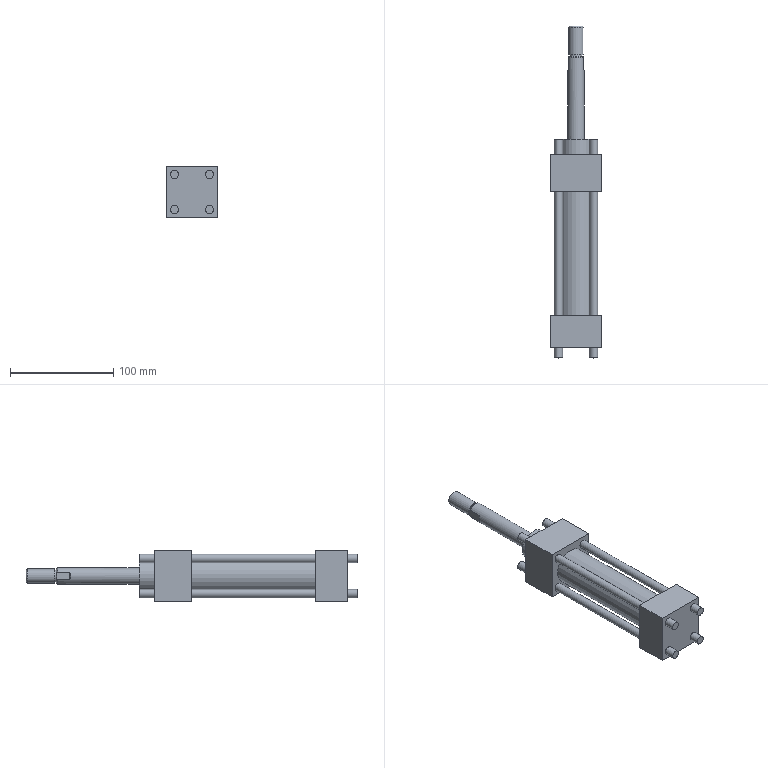Part | NX | features solid 2 | 1 solid | 52 faces | box 50 x 321.5 x 50 mm | volume 339915 mm3 | plane 28 | cylinder 19 | cone 5 | commonest cylinder face diameters 8 x12 15 x2 12 x1 14 x1 16 x1 30 x1
STEP:
#1=CARTESIAN_POINT('',(7.5,-465.5,-35.5));
#2=VERTEX_POINT('',#1);
#3=CARTESIAN_POINT('',(0.,-465.5,-35.5));
#4=DIRECTION('',(0.,0.,-1.));
#5=DIRECTION('',(1.,0.,0.));
#6=AXIS2_PLACEMENT_3D('',#3,#4,#5);
#7=CIRCLE('',#6,7.5);
#8=EDGE_CURVE('',#2,#2,#7,.F.);
#9=ORIENTED_EDGE('',*,*,#8,.T.);
#10=EDGE_LOOP('',(#9));
#11=FACE_BOUND('',#10,.T.);
#12=CARTESIAN_POINT('',(7.5,-465.5,-43.));
#13=VERTEX_POINT('',#12);
#14=CARTESIAN_POINT('',(0.,-465.5,-43.));
#15=DIRECTION('',(0.,0.,1.));
#16=DIRECTION('',(1.,0.,0.));
#17=AXIS2_PLACEMENT_3D('',#14,#15,#16);
#18=CIRCLE('',#17,7.5);
#19=EDGE_CURVE('',#13,#13,#18,.F.);
#20=ORIENTED_EDGE('',*,*,#19,.T.);
#21=EDGE_LOOP('',(#20));
#22=FACE_BOUND('',#21,.T.);
#23=CARTESIAN_POINT('',(0.,-465.5,-45.5));
#24=DIRECTION('',(0.,0.,1.));
#25=DIRECTION('',(1.,0.,0.));
#26=AXIS2_PLACEMENT_3D('',#23,#24,#25);
#27=CYLINDRICAL_SURFACE('',#26,7.5);
#28=ADVANCED_FACE('',(#11,#22),#27,.F.);
#29=CARTESIAN_POINT('',(7.5,-309.5,-35.5));
#30=VERTEX_POINT('',#29);
#31=CARTESIAN_POINT('',(0.,-309.5,-35.5));
#32=DIRECTION('',(0.,0.,-1.));
#33=DIRECTION('',(1.,0.,0.));
#34=AXIS2_PLACEMENT_3D('',#31,#32,#33);
#35=CIRCLE('',#34,7.5);
#36=EDGE_CURVE('',#30,#30,#35,.F.);
#37=ORIENTED_EDGE('',*,*,#36,.T.);
#38=EDGE_LOOP('',(#37));
#39=FACE_BOUND('',#38,.T.);
#40=CARTESIAN_POINT('',(7.5,-309.5,-43.));
#41=VERTEX_POINT('',#40);
#42=CARTESIAN_POINT('',(0.,-309.5,-43.));
#43=DIRECTION('',(0.,0.,1.));
#44=DIRECTION('',(1.,0.,0.));
#45=AXIS2_PLACEMENT_3D('',#42,#43,#44);
#46=CIRCLE('',#45,7.5);
#47=EDGE_CURVE('',#41,#41,#46,.F.);
#48=ORIENTED_EDGE('',*,*,#47,.T.);
#49=EDGE_LOOP('',(#48));
#50=FACE_BOUND('',#49,.T.);
#51=CARTESIAN_POINT('',(0.,-309.5,-45.5));
#52=DIRECTION('',(0.,0.,1.));
#53=DIRECTION('',(1.,0.,0.));
#54=AXIS2_PLACEMENT_3D('',#51,#52,#53);
#55=CYLINDRICAL_SURFACE('',#54,7.5);
#56=ADVANCED_FACE('',(#39,#50),#55,.F.);
#57=CARTESIAN_POINT('',(0.,-167.,-12.));
#58=VERTEX_POINT('',#57);
#59=CARTESIAN_POINT('',(0.,-167.,-18.));
#60=DIRECTION('',(0.,1.,0.));
#61=DIRECTION('',(0.,0.,1.));
#62=AXIS2_PLACEMENT_3D('',#59,#60,#61);
#63=CIRCLE('',#62,6.);
#64=EDGE_CURVE('',#58,#58,#63,.T.);
#65=ORIENTED_EDGE('',*,*,#64,.T.);
#66=EDGE_LOOP('',(#65));
#67=FACE_BOUND('',#66,.T.);
#68=CARTESIAN_POINT('',(0.,-167.,-18.));
#69=DIRECTION('',(0.,1.,0.));
#70=DIRECTION('',(0.,0.,-1.));
#71=AXIS2_PLACEMENT_3D('',#68,#69,#70);
#72=PLANE('',#71);
#73=ADVANCED_FACE('',(#67),#72,.T.);
#74=CARTESIAN_POINT('',(17.,-327.5,-5.));
#75=VERTEX_POINT('',#74);
#76=CARTESIAN_POINT('',(17.,-327.5,-1.));
#77=DIRECTION('',(0.,-1.,0.));
#78=DIRECTION('',(0.,0.,-1.));
#79=AXIS2_PLACEMENT_3D('',#76,#77,#78);
#80=CIRCLE('',#79,4.);
#81=EDGE_CURVE('',#75,#75,#80,.F.);
#82=ORIENTED_EDGE('',*,*,#81,.T.);
#83=EDGE_LOOP('',(#82));
#84=FACE_BOUND('',#83,.T.);
#85=CARTESIAN_POINT('',(17.,-327.5,-39.));
#86=VERTEX_POINT('',#85);
#87=CARTESIAN_POINT('',(17.,-327.5,-35.));
#88=DIRECTION('',(0.,-1.,0.));
#89=DIRECTION('',(0.,0.,-1.));
#90=AXIS2_PLACEMENT_3D('',#87,#88,#89);
#91=CIRCLE('',#90,4.);
#92=EDGE_CURVE('',#86,#86,#91,.F.);
#93=ORIENTED_EDGE('',*,*,#92,.T.);
#94=EDGE_LOOP('',(#93));
#95=FACE_BOUND('',#94,.T.);
#96=CARTESIAN_POINT('',(-17.,-327.5,-5.));
#97=VERTEX_POINT('',#96);
#98=CARTESIAN_POINT('',(-17.,-327.5,-1.));
#99=DIRECTION('',(0.,-1.,0.));
#100=DIRECTION('',(0.,0.,-1.));
#101=AXIS2_PLACEMENT_3D('',#98,#99,#100);
#102=CIRCLE('',#101,4.);
#103=EDGE_CURVE('',#97,#97,#102,.F.);
#104=ORIENTED_EDGE('',*,*,#103,.T.);
#105=EDGE_LOOP('',(#104));
#106=FACE_BOUND('',#105,.T.);
#107=CARTESIAN_POINT('',(-17.,-327.5,-39.));
#108=VERTEX_POINT('',#107);
#109=CARTESIAN_POINT('',(-17.,-327.5,-35.));
#110=DIRECTION('',(0.,-1.,0.));
#111=DIRECTION('',(0.,0.,-1.));
#112=AXIS2_PLACEMENT_3D('',#109,#110,#111);
#113=CIRCLE('',#112,4.);
#114=EDGE_CURVE('',#108,#108,#113,.T.);
#115=ORIENTED_EDGE('',*,*,#114,.F.);
#116=EDGE_LOOP('',(#115));
#117=FACE_BOUND('',#116,.T.);
#118=CARTESIAN_POINT('',(0.,-327.5,-35.5));
#119=VERTEX_POINT('',#118);
#120=CARTESIAN_POINT('',(0.,-327.5,-18.));
#121=DIRECTION('',(0.,-1.,0.));
#122=DIRECTION('',(0.,0.,-1.));
#123=AXIS2_PLACEMENT_3D('',#120,#121,#122);
#124=CIRCLE('',#123,17.5);
#125=EDGE_CURVE('',#119,#119,#124,.F.);
#126=ORIENTED_EDGE('',*,*,#125,.T.);
#127=EDGE_LOOP('',(#126));
#128=FACE_BOUND('',#127,.T.);
#129=CARTESIAN_POINT('',(-25.,-327.5,-43.));
#130=VERTEX_POINT('',#129);
#131=CARTESIAN_POINT('',(-25.,-327.5,7.));
#132=VERTEX_POINT('',#131);
#133=CARTESIAN_POINT('',(-25.,-327.5,9.5));
#134=DIRECTION('',(0.,0.,1.));
#135=VECTOR('',#134,1000.);
#136=LINE('',#133,#135);
#137=EDGE_CURVE('',#130,#132,#136,.T.);
#138=ORIENTED_EDGE('',*,*,#137,.F.);
#139=CARTESIAN_POINT('',(25.,-327.5,-43.));
#140=VERTEX_POINT('',#139);
#141=CARTESIAN_POINT('',(-27.5,-327.5,-43.));
#142=DIRECTION('',(-1.,0.,0.));
#143=VECTOR('',#142,1000.);
#144=LINE('',#141,#143);
#145=EDGE_CURVE('',#140,#130,#144,.T.);
#146=ORIENTED_EDGE('',*,*,#145,.F.);
#147=CARTESIAN_POINT('',(25.,-327.5,7.));
#148=VERTEX_POINT('',#147);
#149=CARTESIAN_POINT('',(25.,-327.5,9.5));
#150=DIRECTION('',(0.,0.,-1.));
#151=VECTOR('',#150,1000.);
#152=LINE('',#149,#151);
#153=EDGE_CURVE('',#148,#140,#152,.T.);
#154=ORIENTED_EDGE('',*,*,#153,.F.);
#155=CARTESIAN_POINT('',(-27.5,-327.5,7.));
#156=DIRECTION('',(1.,0.,0.));
#157=VECTOR('',#156,1000.);
#158=LINE('',#155,#157);
#159=EDGE_CURVE('',#132,#148,#158,.T.);
#160=ORIENTED_EDGE('',*,*,#159,.F.);
#161=EDGE_LOOP('',(#138,#146,#154,#160));
#162=FACE_BOUND('',#161,.T.);
#163=CARTESIAN_POINT('',(-27.5,-327.5,9.5));
#164=DIRECTION('',(0.,-1.,0.));
#165=DIRECTION('',(0.,0.,1.));
#166=AXIS2_PLACEMENT_3D('',#163,#164,#165);
#167=PLANE('',#166);
#168=ADVANCED_FACE('',(#84,#95,#106,#117,#128,#162),#167,.T.);
#169=CARTESIAN_POINT('',(0.,-291.5,-3.));
#170=VERTEX_POINT('',#169);
#171=CARTESIAN_POINT('',(0.,-291.5,-18.));
#172=DIRECTION('',(0.,1.,0.));
#173=DIRECTION('',(0.,0.,1.));
#174=AXIS2_PLACEMENT_3D('',#171,#172,#173);
#175=CIRCLE('',#174,15.);
#176=EDGE_CURVE('',#170,#170,#175,.T.);
#177=ORIENTED_EDGE('',*,*,#176,.F.);
#178=EDGE_LOOP('',(#177));
#179=FACE_BOUND('',#178,.T.);
#180=CARTESIAN_POINT('',(17.,-291.5,-5.));
#181=VERTEX_POINT('',#180);
#182=CARTESIAN_POINT('',(17.,-291.5,-1.));
#183=DIRECTION('',(0.,-1.,0.));
#184=DIRECTION('',(0.,0.,-1.));
#185=AXIS2_PLACEMENT_3D('',#182,#183,#184);
#186=CIRCLE('',#185,4.);
#187=EDGE_CURVE('',#181,#181,#186,.F.);
#188=ORIENTED_EDGE('',*,*,#187,.F.);
#189=EDGE_LOOP('',(#188));
#190=FACE_BOUND('',#189,.T.);
#191=CARTESIAN_POINT('',(17.,-291.5,-39.));
#192=VERTEX_POINT('',#191);
#193=CARTESIAN_POINT('',(17.,-291.5,-35.));
#194=DIRECTION('',(0.,-1.,0.));
#195=DIRECTION('',(0.,0.,-1.));
#196=AXIS2_PLACEMENT_3D('',#193,#194,#195);
#197=CIRCLE('',#196,4.);
#198=EDGE_CURVE('',#192,#192,#197,.F.);
#199=ORIENTED_EDGE('',*,*,#198,.F.);
#200=EDGE_LOOP('',(#199));
#201=FACE_BOUND('',#200,.T.);
#202=CARTESIAN_POINT('',(-17.,-291.5,-5.));
#203=VERTEX_POINT('',#202);
#204=CARTESIAN_POINT('',(-17.,-291.5,-1.));
#205=DIRECTION('',(0.,-1.,0.));
#206=DIRECTION('',(0.,0.,-1.));
#207=AXIS2_PLACEMENT_3D('',#204,#205,#206);
#208=CIRCLE('',#207,4.);
#209=EDGE_CURVE('',#203,#203,#208,.F.);
#210=ORIENTED_EDGE('',*,*,#209,.F.);
#211=EDGE_LOOP('',(#210));
#212=FACE_BOUND('',#211,.T.);
#213=CARTESIAN_POINT('',(-17.,-291.5,-39.));
#214=VERTEX_POINT('',#213);
#215=CARTESIAN_POINT('',(-17.,-291.5,-35.));
#216=DIRECTION('',(0.,-1.,0.));
#217=DIRECTION('',(0.,0.,-1.));
#218=AXIS2_PLACEMENT_3D('',#215,#216,#217);
#219=CIRCLE('',#218,4.);
#220=EDGE_CURVE('',#214,#214,#219,.T.);
#221=ORIENTED_EDGE('',*,*,#220,.T.);
#222=EDGE_LOOP('',(#221));
#223=FACE_BOUND('',#222,.T.);
#224=CARTESIAN_POINT('',(-25.,-291.5,-43.));
#225=VERTEX_POINT('',#224);
#226=CARTESIAN_POINT('',(-25.,-291.5,7.));
#227=VERTEX_POINT('',#226);
#228=CARTESIAN_POINT('',(-25.,-291.5,9.5));
#229=DIRECTION('',(0.,0.,1.));
#230=VECTOR('',#229,1000.);
#231=LINE('',#228,#230);
#232=EDGE_CURVE('',#225,#227,#231,.T.);
#233=ORIENTED_EDGE('',*,*,#232,.T.);
#234=CARTESIAN_POINT('',(25.,-291.5,7.));
#235=VERTEX_POINT('',#234);
#236=CARTESIAN_POINT('',(-27.5,-291.5,7.));
#237=DIRECTION('',(1.,0.,0.));
#238=VECTOR('',#237,1000.);
#239=LINE('',#236,#238);
#240=EDGE_CURVE('',#227,#235,#239,.T.);
#241=ORIENTED_EDGE('',*,*,#240,.T.);
#242=CARTESIAN_POINT('',(25.,-291.5,-43.));
#243=VERTEX_POINT('',#242);
#244=CARTESIAN_POINT('',(25.,-291.5,9.5));
#245=DIRECTION('',(0.,0.,-1.));
#246=VECTOR('',#245,1000.);
#247=LINE('',#244,#246);
#248=EDGE_CURVE('',#235,#243,#247,.T.);
#249=ORIENTED_EDGE('',*,*,#248,.T.);
#250=CARTESIAN_POINT('',(-27.5,-291.5,-43.));
#251=DIRECTION('',(-1.,0.,0.));
#252=VECTOR('',#251,1000.);
#253=LINE('',#250,#252);
#254=EDGE_CURVE('',#243,#225,#253,.T.);
#255=ORIENTED_EDGE('',*,*,#254,.T.);
#256=EDGE_LOOP('',(#233,#241,#249,#255));
#257=FACE_BOUND('',#256,.T.);
#258=CARTESIAN_POINT('',(-27.5,-291.5,9.5));
#259=DIRECTION('',(0.,-1.,0.));
#260=DIRECTION('',(0.,0.,1.));
#261=AXIS2_PLACEMENT_3D('',#258,#259,#260);
#262=PLANE('',#261);
#263=ADVANCED_FACE('',(#179,#190,#201,#212,#223,#257),#262,.F.);
#264=ORIENTED_EDGE('',*,*,#232,.F.);
#265=CARTESIAN_POINT('',(-25.,-327.5,-43.));
#266=DIRECTION('',(0.,1.,0.));
#267=VECTOR('',#266,1000.);
#268=LINE('',#265,#267);
#269=EDGE_CURVE('',#130,#225,#268,.T.);
#270=ORIENTED_EDGE('',*,*,#269,.F.);
#271=ORIENTED_EDGE('',*,*,#137,.T.);
#272=CARTESIAN_POINT('',(-25.,-327.5,7.));
#273=DIRECTION('',(0.,1.,0.));
#274=VECTOR('',#273,1000.);
#275=LINE('',#272,#274);
#276=EDGE_CURVE('',#132,#227,#275,.T.);
#277=ORIENTED_EDGE('',*,*,#276,.T.);
#278=EDGE_LOOP('',(#264,#270,#271,#277));
#279=FACE_BOUND('',#278,.T.);
#280=CARTESIAN_POINT('',(-25.,-327.5,-45.5));
#281=DIRECTION('',(1.,0.,0.));
#282=DIRECTION('',(0.,0.,-1.));
#283=AXIS2_PLACEMENT_3D('',#280,#281,#282);
#284=PLANE('',#283);
#285=ADVANCED_FACE('',(#279),#284,.F.);
#286=ORIENTED_EDGE('',*,*,#240,.F.);
#287=ORIENTED_EDGE('',*,*,#276,.F.);
#288=ORIENTED_EDGE('',*,*,#159,.T.);
#289=CARTESIAN_POINT('',(25.,-327.5,7.));
#290=DIRECTION('',(0.,1.,0.));
#291=VECTOR('',#290,1000.);
#292=LINE('',#289,#291);
#293=EDGE_CURVE('',#148,#235,#292,.T.);
#294=ORIENTED_EDGE('',*,*,#293,.T.);
#295=EDGE_LOOP('',(#286,#287,#288,#294));
#296=FACE_BOUND('',#295,.T.);
#297=CARTESIAN_POINT('',(-27.5,-327.5,7.));
#298=DIRECTION('',(0.,0.,-1.));
#299=DIRECTION('',(0.,-1.,0.));
#300=AXIS2_PLACEMENT_3D('',#297,#298,#299);
#301=PLANE('',#300);
#302=ADVANCED_FACE('',(#296),#301,.F.);
#303=ORIENTED_EDGE('',*,*,#248,.F.);
#304=ORIENTED_EDGE('',*,*,#293,.F.);
#305=ORIENTED_EDGE('',*,*,#153,.T.);
#306=CARTESIAN_POINT('',(25.,-327.5,-43.));
#307=DIRECTION('',(0.,1.,0.));
#308=VECTOR('',#307,1000.);
#309=LINE('',#306,#308);
#310=EDGE_CURVE('',#140,#243,#309,.T.);
#311=ORIENTED_EDGE('',*,*,#310,.T.);
#312=EDGE_LOOP('',(#303,#304,#305,#311));
#313=FACE_BOUND('',#312,.T.);
#314=CARTESIAN_POINT('',(25.,-327.5,9.5));
#315=DIRECTION('',(-1.,0.,0.));
#316=DIRECTION('',(0.,0.,1.));
#317=AXIS2_PLACEMENT_3D('',#314,#315,#316);
#318=PLANE('',#317);
#319=ADVANCED_FACE('',(#313),#318,.F.);
#320=ORIENTED_EDGE('',*,*,#47,.F.);
#321=EDGE_LOOP('',(#320));
#322=FACE_BOUND('',#321,.T.);
#323=ORIENTED_EDGE('',*,*,#254,.F.);
#324=ORIENTED_EDGE('',*,*,#310,.F.);
#325=ORIENTED_EDGE('',*,*,#145,.T.);
#326=ORIENTED_EDGE('',*,*,#269,.T.);
#327=EDGE_LOOP('',(#323,#324,#325,#326));
#328=FACE_BOUND('',#327,.T.);
#329=CARTESIAN_POINT('',(27.5,-327.5,-43.));
#330=DIRECTION('',(0.,0.,1.));
#331=DIRECTION('',(1.,0.,0.));
#332=AXIS2_PLACEMENT_3D('',#329,#330,#331);
#333=PLANE('',#332);
#334=ADVANCED_FACE('',(#322,#328),#333,.F.);
#335=CARTESIAN_POINT('',(0.,-447.5,-35.5));
#336=VERTEX_POINT('',#335);
#337=CARTESIAN_POINT('',(0.,-447.5,-18.));
#338=DIRECTION('',(0.,-1.,0.));
#339=DIRECTION('',(0.,0.,-1.));
#340=AXIS2_PLACEMENT_3D('',#337,#338,#339);
#341=CIRCLE('',#340,17.5);
#342=EDGE_CURVE('',#336,#336,#341,.F.);
#343=ORIENTED_EDGE('',*,*,#342,.T.);
#344=EDGE_LOOP('',(#343));
#345=FACE_BOUND('',#344,.T.);
#346=ORIENTED_EDGE('',*,*,#125,.F.);
#347=EDGE_LOOP('',(#346));
#348=FACE_BOUND('',#347,.T.);
#349=CARTESIAN_POINT('',(0.,-447.5,-18.));
#350=DIRECTION('',(0.,1.,0.));
#351=DIRECTION('',(0.,0.,-1.));
#352=AXIS2_PLACEMENT_3D('',#349,#350,#351);
#353=CYLINDRICAL_SURFACE('',#352,17.5);
#354=ADVANCED_FACE('',(#345,#348),#353,.T.);
#355=ORIENTED_EDGE('',*,*,#36,.F.);
#356=EDGE_LOOP('',(#355));
#357=FACE_BOUND('',#356,.T.);
#358=CARTESIAN_POINT('',(0.,-309.5,-30.994));
#359=VERTEX_POINT('',#358);
#360=VERTEX_LOOP('',#359);
#361=FACE_BOUND('',#360,.T.);
#362=CARTESIAN_POINT('',(0.,-309.5,-35.5));
#363=DIRECTION('',(0.,0.,-1.));
#364=DIRECTION('',(-1.,0.,0.));
#365=AXIS2_PLACEMENT_3D('',#362,#363,#364);
#366=CONICAL_SURFACE('',#365,7.5,1.03);
#367=ADVANCED_FACE('',(#357,#361),#366,.F.);
#368=CARTESIAN_POINT('',(17.,-447.5,-5.));
#369=VERTEX_POINT('',#368);
#370=CARTESIAN_POINT('',(17.,-447.5,-1.));
#371=DIRECTION('',(0.,-1.,0.));
#372=DIRECTION('',(0.,0.,-1.));
#373=AXIS2_PLACEMENT_3D('',#370,#371,#372);
#374=CIRCLE('',#373,4.);
#375=EDGE_CURVE('',#369,#369,#374,.F.);
#376=ORIENTED_EDGE('',*,*,#375,.F.);
#377=EDGE_LOOP('',(#376));
#378=FACE_BOUND('',#377,.T.);
#379=CARTESIAN_POINT('',(17.,-447.5,-39.));
#380=VERTEX_POINT('',#379);
#381=CARTESIAN_POINT('',(17.,-447.5,-35.));
#382=DIRECTION('',(0.,-1.,0.));
#383=DIRECTION('',(0.,0.,-1.));
#384=AXIS2_PLACEMENT_3D('',#381,#382,#383);
#385=CIRCLE('',#384,4.);
#386=EDGE_CURVE('',#380,#380,#385,.F.);
#387=ORIENTED_EDGE('',*,*,#386,.F.);
#388=EDGE_LOOP('',(#387));
#389=FACE_BOUND('',#388,.T.);
#390=CARTESIAN_POINT('',(-17.,-447.5,-5.));
#391=VERTEX_POINT('',#390);
#392=CARTESIAN_POINT('',(-17.,-447.5,-1.));
#393=DIRECTION('',(0.,-1.,0.));
#394=DIRECTION('',(0.,0.,-1.));
#395=AXIS2_PLACEMENT_3D('',#392,#393,#394);
#396=CIRCLE('',#395,4.);
#397=EDGE_CURVE('',#391,#391,#396,.F.);
#398=ORIENTED_EDGE('',*,*,#397,.F.);
#399=EDGE_LOOP('',(#398));
#400=FACE_BOUND('',#399,.T.);
#401=CARTESIAN_POINT('',(-17.,-447.5,-39.));
#402=VERTEX_POINT('',#401);
#403=CARTESIAN_POINT('',(-17.,-447.5,-35.));
#404=DIRECTION('',(0.,-1.,0.));
#405=DIRECTION('',(0.,0.,-1.));
#406=AXIS2_PLACEMENT_3D('',#403,#404,#405);
#407=CIRCLE('',#406,4.);
#408=EDGE_CURVE('',#402,#402,#407,.T.);
#409=ORIENTED_EDGE('',*,*,#408,.T.);
#410=EDGE_LOOP('',(#409));
#411=FACE_BOUND('',#410,.T.);
#412=CARTESIAN_POINT('',(-25.,-447.5,-43.));
#413=VERTEX_POINT('',#412);
#414=CARTESIAN_POINT('',(-25.,-447.5,7.));
#415=VERTEX_POINT('',#414);
#416=CARTESIAN_POINT('',(-25.,-447.5,9.5));
#417=DIRECTION('',(0.,0.,1.));
#418=VECTOR('',#417,1000.);
#419=LINE('',#416,#418);
#420=EDGE_CURVE('',#413,#415,#419,.T.);
#421=ORIENTED_EDGE('',*,*,#420,.T.);
#422=CARTESIAN_POINT('',(25.,-447.5,7.));
#423=VERTEX_POINT('',#422);
#424=CARTESIAN_POINT('',(-27.5,-447.5,7.));
#425=DIRECTION('',(1.,0.,0.));
#426=VECTOR('',#425,1000.);
#427=LINE('',#424,#426);
#428=EDGE_CURVE('',#415,#423,#427,.T.);
#429=ORIENTED_EDGE('',*,*,#428,.T.);
#430=CARTESIAN_POINT('',(25.,-447.5,-43.));
#431=VERTEX_POINT('',#430);
#432=CARTESIAN_POINT('',(25.,-447.5,9.5));
#433=DIRECTION('',(0.,0.,-1.));
#434=VECTOR('',#433,1000.);
#435=LINE('',#432,#434);
#436=EDGE_CURVE('',#423,#431,#435,.T.);
#437=ORIENTED_EDGE('',*,*,#436,.T.);
#438=CARTESIAN_POINT('',(-27.5,-447.5,-43.));
#439=DIRECTION('',(-1.,0.,0.));
#440=VECTOR('',#439,1000.);
#441=LINE('',#438,#440);
#442=EDGE_CURVE('',#431,#413,#441,.T.);
#443=ORIENTED_EDGE('',*,*,#442,.T.);
#444=EDGE_LOOP('',(#421,#429,#437,#443));
#445=FACE_BOUND('',#444,.T.);
#446=ORIENTED_EDGE('',*,*,#342,.F.);
#447=EDGE_LOOP('',(#446));
#448=FACE_BOUND('',#447,.T.);
#449=CARTESIAN_POINT('',(-27.5,-447.5,9.5));
#450=DIRECTION('',(0.,-1.,0.));
#451=DIRECTION('',(0.,0.,1.));
#452=AXIS2_PLACEMENT_3D('',#449,#450,#451);
#453=PLANE('',#452);
#454=ADVANCED_FACE('',(#378,#389,#400,#411,#445,#448),#453,.F.);
#455=CARTESIAN_POINT('',(17.,-478.5,-5.));
#456=VERTEX_POINT('',#455);
#457=CARTESIAN_POINT('',(17.,-478.5,-1.));
#458=DIRECTION('',(0.,-1.,0.));
#459=DIRECTION('',(0.,0.,-1.));
#460=AXIS2_PLACEMENT_3D('',#457,#458,#459);
#461=CIRCLE('',#460,4.);
#462=EDGE_CURVE('',#456,#456,#461,.F.);
#463=ORIENTED_EDGE('',*,*,#462,.T.);
#464=EDGE_LOOP('',(#463));
#465=FACE_BOUND('',#464,.T.);
#466=CARTESIAN_POINT('',(17.,-478.5,-39.));
#467=VERTEX_POINT('',#466);
#468=CARTESIAN_POINT('',(17.,-478.5,-35.));
#469=DIRECTION('',(0.,-1.,0.));
#470=DIRECTION('',(0.,0.,-1.));
#471=AXIS2_PLACEMENT_3D('',#468,#469,#470);
#472=CIRCLE('',#471,4.);
#473=EDGE_CURVE('',#467,#467,#472,.F.);
#474=ORIENTED_EDGE('',*,*,#473,.T.);
#475=EDGE_LOOP('',(#474));
#476=FACE_BOUND('',#475,.T.);
#477=CARTESIAN_POINT('',(-17.,-478.5,-5.));
#478=VERTEX_POINT('',#477);
#479=CARTESIAN_POINT('',(-17.,-478.5,-1.));
#480=DIRECTION('',(0.,-1.,0.));
#481=DIRECTION('',(0.,0.,-1.));
#482=AXIS2_PLACEMENT_3D('',#479,#480,#481);
#483=CIRCLE('',#482,4.);
#484=EDGE_CURVE('',#478,#478,#483,.F.);
#485=ORIENTED_EDGE('',*,*,#484,.T.);
#486=EDGE_LOOP('',(#485));
#487=FACE_BOUND('',#486,.T.);
#488=CARTESIAN_POINT('',(-17.,-478.5,-39.));
#489=VERTEX_POINT('',#488);
#490=CARTESIAN_POINT('',(-17.,-478.5,-35.));
#491=DIRECTION('',(0.,-1.,0.));
#492=DIRECTION('',(0.,0.,-1.));
#493=AXIS2_PLACEMENT_3D('',#490,#491,#492);
#494=CIRCLE('',#493,4.);
#495=EDGE_CURVE('',#489,#489,#494,.T.);
#496=ORIENTED_EDGE('',*,*,#495,.F.);
#497=EDGE_LOOP('',(#496));
#498=FACE_BOUND('',#497,.T.);
#499=CARTESIAN_POINT('',(25.,-478.5,7.));
#500=VERTEX_POINT('',#499);
#501=CARTESIAN_POINT('',(25.,-478.5,-43.));
#502=VERTEX_POINT('',#501);
#503=CARTESIAN_POINT('',(25.,-478.5,9.5));
#504=DIRECTION('',(0.,0.,-1.));
#505=VECTOR('',#504,1000.);
#506=LINE('',#503,#505);
#507=EDGE_CURVE('',#500,#502,#506,.T.);
#508=ORIENTED_EDGE('',*,*,#507,.F.);
#509=CARTESIAN_POINT('',(-25.,-478.5,7.));
#510=VERTEX_POINT('',#509);
#511=CARTESIAN_POINT('',(-27.5,-478.5,7.));
#512=DIRECTION('',(1.,0.,0.));
#513=VECTOR('',#512,1000.);
#514=LINE('',#511,#513);
#515=EDGE_CURVE('',#510,#500,#514,.T.);
#516=ORIENTED_EDGE('',*,*,#515,.F.);
#517=CARTESIAN_POINT('',(-25.,-478.5,-43.));
#518=VERTEX_POINT('',#517);
#519=CARTESIAN_POINT('',(-25.,-478.5,9.5));
#520=DIRECTION('',(0.,0.,1.));
#521=VECTOR('',#520,1000.);
#522=LINE('',#519,#521);
#523=EDGE_CURVE('',#518,#510,#522,.T.);
#524=ORIENTED_EDGE('',*,*,#523,.F.);
#525=CARTESIAN_POINT('',(-27.5,-478.5,-43.));
#526=DIRECTION('',(-1.,0.,0.));
#527=VECTOR('',#526,1000.);
#528=LINE('',#525,#527);
#529=EDGE_CURVE('',#502,#518,#528,.T.);
#530=ORIENTED_EDGE('',*,*,#529,.F.);
#531=EDGE_LOOP('',(#508,#516,#524,#530));
#532=FACE_BOUND('',#531,.T.);
#533=CARTESIAN_POINT('',(-27.5,-478.5,9.5));
#534=DIRECTION('',(0.,-1.,0.));
#535=DIRECTION('',(0.,0.,1.));
#536=AXIS2_PLACEMENT_3D('',#533,#534,#535);
#537=PLANE('',#536);
#538=ADVANCED_FACE('',(#465,#476,#487,#498,#532),#537,.T.);
#539=ORIENTED_EDGE('',*,*,#420,.F.);
#540=CARTESIAN_POINT('',(-25.,-478.5,-43.));
#541=DIRECTION('',(0.,1.,0.));
#542=VECTOR('',#541,1000.);
#543=LINE('',#540,#542);
#544=EDGE_CURVE('',#518,#413,#543,.T.);
#545=ORIENTED_EDGE('',*,*,#544,.F.);
#546=ORIENTED_EDGE('',*,*,#523,.T.);
#547=CARTESIAN_POINT('',(-25.,-478.5,7.));
#548=DIRECTION('',(0.,1.,0.));
#549=VECTOR('',#548,1000.);
#550=LINE('',#547,#549);
#551=EDGE_CURVE('',#510,#415,#550,.T.);
#552=ORIENTED_EDGE('',*,*,#551,.T.);
#553=EDGE_LOOP('',(#539,#545,#546,#552));
#554=FACE_BOUND('',#553,.T.);
#555=CARTESIAN_POINT('',(-25.,-478.5,-45.5));
#556=DIRECTION('',(1.,0.,0.));
#557=DIRECTION('',(0.,0.,-1.));
#558=AXIS2_PLACEMENT_3D('',#555,#556,#557);
#559=PLANE('',#558);
#560=ADVANCED_FACE('',(#554),#559,.F.);
#561=ORIENTED_EDGE('',*,*,#428,.F.);
#562=ORIENTED_EDGE('',*,*,#551,.F.);
#563=ORIENTED_EDGE('',*,*,#515,.T.);
#564=CARTESIAN_POINT('',(25.,-478.5,7.));
#565=DIRECTION('',(0.,1.,0.));
#566=VECTOR('',#565,1000.);
#567=LINE('',#564,#566);
#568=EDGE_CURVE('',#500,#423,#567,.T.);
#569=ORIENTED_EDGE('',*,*,#568,.T.);
#570=EDGE_LOOP('',(#561,#562,#563,#569));
#571=FACE_BOUND('',#570,.T.);
#572=CARTESIAN_POINT('',(-27.5,-478.5,7.));
#573=DIRECTION('',(0.,0.,-1.));
#574=DIRECTION('',(-1.,0.,0.));
#575=AXIS2_PLACEMENT_3D('',#572,#573,#574);
#576=PLANE('',#575);
#577=ADVANCED_FACE('',(#571),#576,.F.);
#578=ORIENTED_EDGE('',*,*,#436,.F.);
#579=ORIENTED_EDGE('',*,*,#568,.F.);
#580=ORIENTED_EDGE('',*,*,#507,.T.);
#581=CARTESIAN_POINT('',(25.,-478.5,-43.));
#582=DIRECTION('',(0.,1.,0.));
#583=VECTOR('',#582,1000.);
#584=LINE('',#581,#583);
#585=EDGE_CURVE('',#502,#431,#584,.T.);
#586=ORIENTED_EDGE('',*,*,#585,.T.);
#587=EDGE_LOOP('',(#578,#579,#580,#586));
#588=FACE_BOUND('',#587,.T.);
#589=CARTESIAN_POINT('',(25.,-478.5,9.5));
#590=DIRECTION('',(-1.,0.,0.));
#591=DIRECTION('',(0.,0.,1.));
#592=AXIS2_PLACEMENT_3D('',#589,#590,#591);
#593=PLANE('',#592);
#594=ADVANCED_FACE('',(#588),#593,.F.);
#595=ORIENTED_EDGE('',*,*,#19,.F.);
#596=EDGE_LOOP('',(#595));
#597=FACE_BOUND('',#596,.T.);
#598=ORIENTED_EDGE('',*,*,#442,.F.);
#599=ORIENTED_EDGE('',*,*,#585,.F.);
#600=ORIENTED_EDGE('',*,*,#529,.T.);
#601=ORIENTED_EDGE('',*,*,#544,.T.);
#602=EDGE_LOOP('',(#598,#599,#600,#601));
#603=FACE_BOUND('',#602,.T.);
#604=CARTESIAN_POINT('',(27.5,-478.5,-43.));
#605=DIRECTION('',(0.,0.,1.));
#606=DIRECTION('',(1.,0.,0.));
#607=AXIS2_PLACEMENT_3D('',#604,#605,#606);
#608=PLANE('',#607);
#609=ADVANCED_FACE('',(#597,#603),#608,.F.);
#610=ORIENTED_EDGE('',*,*,#8,.F.);
#611=EDGE_LOOP('',(#610));
#612=FACE_BOUND('',#611,.T.);
#613=CARTESIAN_POINT('',(0.,-465.5,-30.994));
#614=VERTEX_POINT('',#613);
#615=VERTEX_LOOP('',#614);
#616=FACE_BOUND('',#615,.T.);
#617=CARTESIAN_POINT('',(0.,-465.5,-35.5));
#618=DIRECTION('',(0.,0.,-1.));
#619=DIRECTION('',(-1.,0.,0.));
#620=AXIS2_PLACEMENT_3D('',#617,#618,#619);
#621=CONICAL_SURFACE('',#620,7.5,1.03);
#622=ADVANCED_FACE('',(#612,#616),#621,.F.);
#623=CARTESIAN_POINT('',(-17.,-488.5,-31.));
#624=VERTEX_POINT('',#623);
#625=CARTESIAN_POINT('',(-17.,-488.5,-35.));
#626=DIRECTION('',(0.,1.,0.));
#627=DIRECTION('',(0.,0.,1.));
#628=AXIS2_PLACEMENT_3D('',#625,#626,#627);
#629=CIRCLE('',#628,4.);
#630=EDGE_CURVE('',#624,#624,#629,.T.);
#631=ORIENTED_EDGE('',*,*,#630,.F.);
#632=EDGE_LOOP('',(#631));
#633=FACE_BOUND('',#632,.T.);
#634=CARTESIAN_POINT('',(20.,-488.5,-38.));
#635=DIRECTION('',(0.,1.,0.));
#636=DIRECTION('',(0.,0.,-1.));
#637=AXIS2_PLACEMENT_3D('',#634,#635,#636);
#638=PLANE('',#637);
#639=ADVANCED_FACE('',(#633),#638,.F.);
#640=ORIENTED_EDGE('',*,*,#495,.T.);
#641=EDGE_LOOP('',(#640));
#642=FACE_BOUND('',#641,.T.);
#643=ORIENTED_EDGE('',*,*,#630,.T.);
#644=EDGE_LOOP('',(#643));
#645=FACE_BOUND('',#644,.T.);
#646=CARTESIAN_POINT('',(-17.,-561.5,-35.));
#647=DIRECTION('',(0.,1.,0.));
#648=DIRECTION('',(0.,0.,1.));
#649=AXIS2_PLACEMENT_3D('',#646,#647,#648);
#650=CYLINDRICAL_SURFACE('',#649,4.);
#651=ADVANCED_FACE('',(#642,#645),#650,.T.);
#652=ORIENTED_EDGE('',*,*,#114,.T.);
#653=EDGE_LOOP('',(#652));
#654=FACE_BOUND('',#653,.T.);
#655=ORIENTED_EDGE('',*,*,#408,.F.);
#656=EDGE_LOOP('',(#655));
#657=FACE_BOUND('',#656,.T.);
#658=CARTESIAN_POINT('',(-17.,-556.5,-35.));
#659=DIRECTION('',(0.,1.,0.));
#660=DIRECTION('',(0.,0.,1.));
#661=AXIS2_PLACEMENT_3D('',#658,#659,#660);
#662=CYLINDRICAL_SURFACE('',#661,4.);
#663=ADVANCED_FACE('',(#654,#657),#662,.T.);
#664=CARTESIAN_POINT('',(-17.,-276.5,-31.));
#665=VERTEX_POINT('',#664);
#666=CARTESIAN_POINT('',(-17.,-276.5,-35.));
#667=DIRECTION('',(0.,1.,0.));
#668=DIRECTION('',(0.,0.,1.));
#669=AXIS2_PLACEMENT_3D('',#666,#667,#668);
#670=CIRCLE('',#669,4.);
#671=EDGE_CURVE('',#665,#665,#670,.T.);
#672=ORIENTED_EDGE('',*,*,#671,.F.);
#673=EDGE_LOOP('',(#672));
#674=FACE_BOUND('',#673,.T.);
#675=ORIENTED_EDGE('',*,*,#220,.F.);
#676=EDGE_LOOP('',(#675));
#677=FACE_BOUND('',#676,.T.);
#678=CARTESIAN_POINT('',(-17.,-556.5,-35.));
#679=DIRECTION('',(0.,1.,0.));
#680=DIRECTION('',(0.,0.,1.));
#681=AXIS2_PLACEMENT_3D('',#678,#679,#680);
#682=CYLINDRICAL_SURFACE('',#681,4.);
#683=ADVANCED_FACE('',(#674,#677),#682,.T.);
#684=ORIENTED_EDGE('',*,*,#671,.T.);
#685=EDGE_LOOP('',(#684));
#686=FACE_BOUND('',#685,.T.);
#687=CARTESIAN_POINT('',(-17.,-276.5,-35.));
#688=DIRECTION('',(0.,1.,0.));
#689=DIRECTION('',(0.,0.,1.));
#690=AXIS2_PLACEMENT_3D('',#687,#688,#689);
#691=PLANE('',#690);
#692=ADVANCED_FACE('',(#686),#691,.T.);
#693=CARTESIAN_POINT('',(-17.,-488.5,3.));
#694=VERTEX_POINT('',#693);
#695=CARTESIAN_POINT('',(-17.,-488.5,-1.));
#696=DIRECTION('',(0.,1.,0.));
#697=DIRECTION('',(0.,0.,1.));
#698=AXIS2_PLACEMENT_3D('',#695,#696,#697);
#699=CIRCLE('',#698,4.);
#700=EDGE_CURVE('',#694,#694,#699,.F.);
#701=ORIENTED_EDGE('',*,*,#700,.T.);
#702=EDGE_LOOP('',(#701));
#703=FACE_BOUND('',#702,.T.);
#704=CARTESIAN_POINT('',(20.,-488.5,-38.));
#705=DIRECTION('',(0.,1.,0.));
#706=DIRECTION('',(0.,0.,-1.));
#707=AXIS2_PLACEMENT_3D('',#704,#705,#706);
#708=PLANE('',#707);
#709=ADVANCED_FACE('',(#703),#708,.F.);
#710=ORIENTED_EDGE('',*,*,#484,.F.);
#711=EDGE_LOOP('',(#710));
#712=FACE_BOUND('',#711,.T.);
#713=ORIENTED_EDGE('',*,*,#700,.F.);
#714=EDGE_LOOP('',(#713));
#715=FACE_BOUND('',#714,.T.);
#716=CARTESIAN_POINT('',(-17.,-561.5,-1.));
#717=DIRECTION('',(0.,1.,0.));
#718=DIRECTION('',(0.,0.,1.));
#719=AXIS2_PLACEMENT_3D('',#716,#717,#718);
#720=CYLINDRICAL_SURFACE('',#719,4.);
#721=ADVANCED_FACE('',(#712,#715),#720,.T.);
#722=ORIENTED_EDGE('',*,*,#103,.F.);
#723=EDGE_LOOP('',(#722));
#724=FACE_BOUND('',#723,.T.);
#725=ORIENTED_EDGE('',*,*,#397,.T.);
#726=EDGE_LOOP('',(#725));
#727=FACE_BOUND('',#726,.T.);
#728=CARTESIAN_POINT('',(-17.,-556.5,-1.));
#729=DIRECTION('',(0.,1.,0.));
#730=DIRECTION('',(0.,0.,1.));
#731=AXIS2_PLACEMENT_3D('',#728,#729,#730);
#732=CYLINDRICAL_SURFACE('',#731,4.);
#733=ADVANCED_FACE('',(#724,#727),#732,.T.);
#734=CARTESIAN_POINT('',(-17.,-276.5,-5.));
#735=VERTEX_POINT('',#734);
#736=CARTESIAN_POINT('',(-17.,-276.5,-1.));
#737=DIRECTION('',(0.,-1.,0.));
#738=DIRECTION('',(0.,0.,-1.));
#739=AXIS2_PLACEMENT_3D('',#736,#737,#738);
#740=CIRCLE('',#739,4.);
#741=EDGE_CURVE('',#735,#735,#740,.T.);
#742=ORIENTED_EDGE('',*,*,#741,.T.);
#743=EDGE_LOOP('',(#742));
#744=FACE_BOUND('',#743,.T.);
#745=ORIENTED_EDGE('',*,*,#209,.T.);
#746=EDGE_LOOP('',(#745));
#747=FACE_BOUND('',#746,.T.);
#748=CARTESIAN_POINT('',(-17.,-556.5,-1.));
#749=DIRECTION('',(0.,1.,0.));
#750=DIRECTION('',(0.,0.,1.));
#751=AXIS2_PLACEMENT_3D('',#748,#749,#750);
#752=CYLINDRICAL_SURFACE('',#751,4.);
#753=ADVANCED_FACE('',(#744,#747),#752,.T.);
#754=ORIENTED_EDGE('',*,*,#741,.F.);
#755=EDGE_LOOP('',(#754));
#756=FACE_BOUND('',#755,.T.);
#757=CARTESIAN_POINT('',(-17.,-276.5,-1.));
#758=DIRECTION('',(0.,-1.,0.));
#759=DIRECTION('',(0.,0.,-1.));
#760=AXIS2_PLACEMENT_3D('',#757,#758,#759);
#761=PLANE('',#760);
#762=ADVANCED_FACE('',(#756),#761,.F.);
#763=CARTESIAN_POINT('',(17.,-488.5,-39.));
#764=VERTEX_POINT('',#763);
#765=CARTESIAN_POINT('',(17.,-488.5,-35.));
#766=DIRECTION('',(0.,-1.,0.));
#767=DIRECTION('',(0.,0.,-1.));
#768=AXIS2_PLACEMENT_3D('',#765,#766,#767);
#769=CIRCLE('',#768,4.);
#770=EDGE_CURVE('',#764,#764,#769,.T.);
#771=ORIENTED_EDGE('',*,*,#770,.T.);
#772=EDGE_LOOP('',(#771));
#773=FACE_BOUND('',#772,.T.);
#774=CARTESIAN_POINT('',(20.,-488.5,2.));
#775=DIRECTION('',(0.,-1.,0.));
#776=DIRECTION('',(0.,0.,1.));
#777=AXIS2_PLACEMENT_3D('',#774,#775,#776);
#778=PLANE('',#777);
#779=ADVANCED_FACE('',(#773),#778,.T.);
#780=ORIENTED_EDGE('',*,*,#473,.F.);
#781=EDGE_LOOP('',(#780));
#782=FACE_BOUND('',#781,.T.);
#783=ORIENTED_EDGE('',*,*,#770,.F.);
#784=EDGE_LOOP('',(#783));
#785=FACE_BOUND('',#784,.T.);
#786=CARTESIAN_POINT('',(17.,-561.5,-35.));
#787=DIRECTION('',(0.,1.,0.));
#788=DIRECTION('',(0.,0.,1.));
#789=AXIS2_PLACEMENT_3D('',#786,#787,#788);
#790=CYLINDRICAL_SURFACE('',#789,4.);
#791=ADVANCED_FACE('',(#782,#785),#790,.T.);
#792=ORIENTED_EDGE('',*,*,#92,.F.);
#793=EDGE_LOOP('',(#792));
#794=FACE_BOUND('',#793,.T.);
#795=ORIENTED_EDGE('',*,*,#386,.T.);
#796=EDGE_LOOP('',(#795));
#797=FACE_BOUND('',#796,.T.);
#798=CARTESIAN_POINT('',(17.,-556.5,-35.));
#799=DIRECTION('',(0.,1.,0.));
#800=DIRECTION('',(0.,0.,1.));
#801=AXIS2_PLACEMENT_3D('',#798,#799,#800);
#802=CYLINDRICAL_SURFACE('',#801,4.);
#803=ADVANCED_FACE('',(#794,#797),#802,.T.);
#804=CARTESIAN_POINT('',(17.,-276.5,-39.));
#805=VERTEX_POINT('',#804);
#806=CARTESIAN_POINT('',(17.,-276.5,-35.));
#807=DIRECTION('',(0.,-1.,0.));
#808=DIRECTION('',(0.,0.,-1.));
#809=AXIS2_PLACEMENT_3D('',#806,#807,#808);
#810=CIRCLE('',#809,4.);
#811=EDGE_CURVE('',#805,#805,#810,.T.);
#812=ORIENTED_EDGE('',*,*,#811,.T.);
#813=EDGE_LOOP('',(#812));
#814=FACE_BOUND('',#813,.T.);
#815=ORIENTED_EDGE('',*,*,#198,.T.);
#816=EDGE_LOOP('',(#815));
#817=FACE_BOUND('',#816,.T.);
#818=CARTESIAN_POINT('',(17.,-556.5,-35.));
#819=DIRECTION('',(0.,1.,0.));
#820=DIRECTION('',(0.,0.,1.));
#821=AXIS2_PLACEMENT_3D('',#818,#819,#820);
#822=CYLINDRICAL_SURFACE('',#821,4.);
#823=ADVANCED_FACE('',(#814,#817),#822,.T.);
#824=ORIENTED_EDGE('',*,*,#811,.F.);
#825=EDGE_LOOP('',(#824));
#826=FACE_BOUND('',#825,.T.);
#827=CARTESIAN_POINT('',(17.,-276.5,-35.));
#828=DIRECTION('',(0.,-1.,0.));
#829=DIRECTION('',(0.,0.,-1.));
#830=AXIS2_PLACEMENT_3D('',#827,#828,#829);
#831=PLANE('',#830);
#832=ADVANCED_FACE('',(#826),#831,.F.);
#833=CARTESIAN_POINT('',(17.,-488.5,-5.));
#834=VERTEX_POINT('',#833);
#835=CARTESIAN_POINT('',(17.,-488.5,-1.));
#836=DIRECTION('',(0.,-1.,0.));
#837=DIRECTION('',(0.,0.,-1.));
#838=AXIS2_PLACEMENT_3D('',#835,#836,#837);
#839=CIRCLE('',#838,4.);
#840=EDGE_CURVE('',#834,#834,#839,.T.);
#841=ORIENTED_EDGE('',*,*,#840,.T.);
#842=EDGE_LOOP('',(#841));
#843=FACE_BOUND('',#842,.T.);
#844=CARTESIAN_POINT('',(20.,-488.5,2.));
#845=DIRECTION('',(0.,-1.,0.));
#846=DIRECTION('',(0.,0.,1.));
#847=AXIS2_PLACEMENT_3D('',#844,#845,#846);
#848=PLANE('',#847);
#849=ADVANCED_FACE('',(#843),#848,.T.);
#850=ORIENTED_EDGE('',*,*,#462,.F.);
#851=EDGE_LOOP('',(#850));
#852=FACE_BOUND('',#851,.T.);
#853=ORIENTED_EDGE('',*,*,#840,.F.);
#854=EDGE_LOOP('',(#853));
#855=FACE_BOUND('',#854,.T.);
#856=CARTESIAN_POINT('',(17.,-561.5,-1.));
#857=DIRECTION('',(0.,1.,0.));
#858=DIRECTION('',(0.,0.,1.));
#859=AXIS2_PLACEMENT_3D('',#856,#857,#858);
#860=CYLINDRICAL_SURFACE('',#859,4.);
#861=ADVANCED_FACE('',(#852,#855),#860,.T.);
#862=ORIENTED_EDGE('',*,*,#81,.F.);
#863=EDGE_LOOP('',(#862));
#864=FACE_BOUND('',#863,.T.);
#865=ORIENTED_EDGE('',*,*,#375,.T.);
#866=EDGE_LOOP('',(#865));
#867=FACE_BOUND('',#866,.T.);
#868=CARTESIAN_POINT('',(17.,-556.5,-1.));
#869=DIRECTION('',(0.,1.,0.));
#870=DIRECTION('',(0.,0.,1.));
#871=AXIS2_PLACEMENT_3D('',#868,#869,#870);
#872=CYLINDRICAL_SURFACE('',#871,4.);
#873=ADVANCED_FACE('',(#864,#867),#872,.T.);
#874=CARTESIAN_POINT('',(17.,-276.5,-5.));
#875=VERTEX_POINT('',#874);
#876=CARTESIAN_POINT('',(17.,-276.5,-1.));
#877=DIRECTION('',(0.,-1.,0.));
#878=DIRECTION('',(0.,0.,-1.));
#879=AXIS2_PLACEMENT_3D('',#876,#877,#878);
#880=CIRCLE('',#879,4.);
#881=EDGE_CURVE('',#875,#875,#880,.T.);
#882=ORIENTED_EDGE('',*,*,#881,.T.);
#883=EDGE_LOOP('',(#882));
#884=FACE_BOUND('',#883,.T.);
#885=ORIENTED_EDGE('',*,*,#187,.T.);
#886=EDGE_LOOP('',(#885));
#887=FACE_BOUND('',#886,.T.);
#888=CARTESIAN_POINT('',(17.,-556.5,-1.));
#889=DIRECTION('',(0.,1.,0.));
#890=DIRECTION('',(0.,0.,1.));
#891=AXIS2_PLACEMENT_3D('',#888,#889,#890);
#892=CYLINDRICAL_SURFACE('',#891,4.);
#893=ADVANCED_FACE('',(#884,#887),#892,.T.);
#894=ORIENTED_EDGE('',*,*,#881,.F.);
#895=EDGE_LOOP('',(#894));
#896=FACE_BOUND('',#895,.T.);
#897=CARTESIAN_POINT('',(17.,-276.5,-1.));
#898=DIRECTION('',(0.,-1.,0.));
#899=DIRECTION('',(0.,0.,-1.));
#900=AXIS2_PLACEMENT_3D('',#897,#898,#899);
#901=PLANE('',#900);
#902=ADVANCED_FACE('',(#896),#901,.F.);
#903=CARTESIAN_POINT('',(0.,-168.,-11.));
#904=VERTEX_POINT('',#903);
#905=CARTESIAN_POINT('',(0.,-168.,-18.));
#906=DIRECTION('',(0.,1.,0.));
#907=DIRECTION('',(0.,0.,1.));
#908=AXIS2_PLACEMENT_3D('',#905,#906,#907);
#909=CIRCLE('',#908,7.);
#910=EDGE_CURVE('',#904,#904,#909,.F.);
#911=ORIENTED_EDGE('',*,*,#910,.T.);
#912=EDGE_LOOP('',(#911));
#913=FACE_BOUND('',#912,.T.);
#914=CARTESIAN_POINT('',(0.,-195.,-25.));
#915=VERTEX_POINT('',#914);
#916=CARTESIAN_POINT('',(0.,-195.,-18.));
#917=DIRECTION('',(0.,-1.,0.));
#918=DIRECTION('',(0.,0.,-1.));
#919=AXIS2_PLACEMENT_3D('',#916,#917,#918);
#920=CIRCLE('',#919,7.);
#921=EDGE_CURVE('',#915,#915,#920,.T.);
#922=ORIENTED_EDGE('',*,*,#921,.F.);
#923=EDGE_LOOP('',(#922));
#924=FACE_BOUND('',#923,.T.);
#925=CARTESIAN_POINT('',(0.,-195.,-18.));
#926=DIRECTION('',(0.,1.,0.));
#927=DIRECTION('',(0.,0.,-1.));
#928=AXIS2_PLACEMENT_3D('',#925,#926,#927);
#929=CYLINDRICAL_SURFACE('',#928,7.);
#930=ADVANCED_FACE('',(#913,#924),#929,.T.);
#931=ORIENTED_EDGE('',*,*,#921,.T.);
#932=EDGE_LOOP('',(#931));
#933=FACE_BOUND('',#932,.T.);
#934=CARTESIAN_POINT('',(0.,-195.,-24.));
#935=VERTEX_POINT('',#934);
#936=CARTESIAN_POINT('',(0.,-195.,-18.));
#937=DIRECTION('',(0.,-1.,0.));
#938=DIRECTION('',(0.,0.,-1.));
#939=AXIS2_PLACEMENT_3D('',#936,#937,#938);
#940=CIRCLE('',#939,6.);
#941=EDGE_CURVE('',#935,#935,#940,.F.);
#942=ORIENTED_EDGE('',*,*,#941,.T.);
#943=EDGE_LOOP('',(#942));
#944=FACE_BOUND('',#943,.T.);
#945=CARTESIAN_POINT('',(0.,-195.,-18.));
#946=DIRECTION('',(0.,-1.,0.));
#947=DIRECTION('',(0.,0.,1.));
#948=AXIS2_PLACEMENT_3D('',#945,#946,#947);
#949=PLANE('',#948);
#950=ADVANCED_FACE('',(#933,#944),#949,.T.);
#951=ORIENTED_EDGE('',*,*,#941,.F.);
#952=EDGE_LOOP('',(#951));
#953=FACE_BOUND('',#952,.T.);
#954=CARTESIAN_POINT('',(0.,-196.5,-12.));
#955=VERTEX_POINT('',#954);
#956=CARTESIAN_POINT('',(0.,-196.5,-18.));
#957=DIRECTION('',(0.,1.,0.));
#958=DIRECTION('',(0.,0.,1.));
#959=AXIS2_PLACEMENT_3D('',#956,#957,#958);
#960=CIRCLE('',#959,6.);
#961=EDGE_CURVE('',#955,#955,#960,.F.);
#962=ORIENTED_EDGE('',*,*,#961,.F.);
#963=EDGE_LOOP('',(#962));
#964=FACE_BOUND('',#963,.T.);
#965=CARTESIAN_POINT('',(0.,-196.5,-18.));
#966=DIRECTION('',(0.,1.,0.));
#967=DIRECTION('',(0.,0.,-1.));
#968=AXIS2_PLACEMENT_3D('',#965,#966,#967);
#969=CYLINDRICAL_SURFACE('',#968,6.);
#970=ADVANCED_FACE('',(#953,#964),#969,.T.);
#971=ORIENTED_EDGE('',*,*,#961,.T.);
#972=EDGE_LOOP('',(#971));
#973=FACE_BOUND('',#972,.T.);
#974=CARTESIAN_POINT('',(7.,-196.5,-18.));
#975=VERTEX_POINT('',#974);
#976=CARTESIAN_POINT('',(-7.,-196.5,-18.));
#977=VERTEX_POINT('',#976);
#978=CARTESIAN_POINT('',(0.,-196.5,-18.));
#979=DIRECTION('',(0.,-1.,0.));
#980=DIRECTION('',(0.,0.,-1.));
#981=AXIS2_PLACEMENT_3D('',#978,#979,#980);
#982=CIRCLE('',#981,7.);
#983=EDGE_CURVE('',#975,#977,#982,.T.);
#984=ORIENTED_EDGE('',*,*,#983,.F.);
#985=CARTESIAN_POINT('',(0.,-196.5,-18.));
#986=DIRECTION('',(0.,-1.,0.));
#987=DIRECTION('',(0.,0.,-1.));
#988=AXIS2_PLACEMENT_3D('',#985,#986,#987);
#989=CIRCLE('',#988,7.);
#990=EDGE_CURVE('',#977,#975,#989,.T.);
#991=ORIENTED_EDGE('',*,*,#990,.F.);
#992=EDGE_LOOP('',(#984,#991));
#993=FACE_BOUND('',#992,.T.);
#994=CARTESIAN_POINT('',(0.,-196.5,-18.));
#995=DIRECTION('',(0.,1.,0.));
#996=DIRECTION('',(0.,0.,-1.));
#997=AXIS2_PLACEMENT_3D('',#994,#995,#996);
#998=PLANE('',#997);
#999=ADVANCED_FACE('',(#973,#993),#998,.T.);
#1000=CARTESIAN_POINT('',(-7.,-209.5,-14.127));
#1001=VERTEX_POINT('',#1000);
#1002=CARTESIAN_POINT('',(-7.,-209.5,-21.873));
#1003=VERTEX_POINT('',#1002);
#1004=CARTESIAN_POINT('',(-7.,-209.5,-26.));
#1005=DIRECTION('',(0.,0.,1.));
#1006=VECTOR('',#1005,1000.);
#1007=LINE('',#1004,#1006);
#1008=EDGE_CURVE('',#1001,#1003,#1007,.F.);
#1009=ORIENTED_EDGE('',*,*,#1008,.T.);
#1010=CARTESIAN_POINT('',(0.,-202.5,-18.));
#1011=DIRECTION('',(0.7071,-0.7071,0.));
#1012=DIRECTION('',(0.7071,0.7071,0.));
#1013=AXIS2_PLACEMENT_3D('',#1010,#1011,#1012);
#1014=ELLIPSE('',#1013,11.314,8.);
#1015=EDGE_CURVE('',#1003,#1001,#1014,.F.);
#1016=ORIENTED_EDGE('',*,*,#1015,.T.);
#1017=EDGE_LOOP('',(#1009,#1016));
#1018=FACE_BOUND('',#1017,.T.);
#1019=CARTESIAN_POINT('',(-8.,-210.5,-26.));
#1020=DIRECTION('',(-0.7071,0.7071,0.));
#1021=DIRECTION('',(-0.7071,-0.7071,0.));
#1022=AXIS2_PLACEMENT_3D('',#1019,#1020,#1021);
#1023=PLANE('',#1022);
#1024=ADVANCED_FACE('',(#1018),#1023,.T.);
#1025=CARTESIAN_POINT('',(-7.,-197.5,-21.873));
#1026=VERTEX_POINT('',#1025);
#1027=CARTESIAN_POINT('',(-7.,-196.5,-18.));
#1028=CARTESIAN_POINT('',(-7.,-196.5,-19.357));
#1029=CARTESIAN_POINT('',(-7.,-196.918,-20.671));
#1030=CARTESIAN_POINT('',(-7.,-197.5,-21.873));
#1031=B_SPLINE_CURVE_WITH_KNOTS('',3,(#1027,#1028,#1029,#1030),.UNSPECIFIED.,.F.,.F.,(4,4),(0.02413,0.02812),.UNSPECIFIED.);
#1032=EDGE_CURVE('',#977,#1026,#1031,.T.);
#1033=ORIENTED_EDGE('',*,*,#1032,.T.);
#1034=CARTESIAN_POINT('',(-7.,-212.5,-21.873));
#1035=DIRECTION('',(0.,1.,0.));
#1036=VECTOR('',#1035,1000.);
#1037=LINE('',#1034,#1036);
#1038=EDGE_CURVE('',#1026,#1003,#1037,.F.);
#1039=ORIENTED_EDGE('',*,*,#1038,.T.);
#1040=ORIENTED_EDGE('',*,*,#1008,.F.);
#1041=CARTESIAN_POINT('',(-7.,-197.5,-14.127));
#1042=VERTEX_POINT('',#1041);
#1043=CARTESIAN_POINT('',(-7.,-212.5,-14.127));
#1044=DIRECTION('',(0.,1.,0.));
#1045=VECTOR('',#1044,1000.);
#1046=LINE('',#1043,#1045);
#1047=EDGE_CURVE('',#1001,#1042,#1046,.T.);
#1048=ORIENTED_EDGE('',*,*,#1047,.T.);
#1049=CARTESIAN_POINT('',(-7.,-197.5,-14.127));
#1050=CARTESIAN_POINT('',(-7.,-196.922,-15.321));
#1051=CARTESIAN_POINT('',(-7.,-196.5,-16.64));
#1052=CARTESIAN_POINT('',(-7.,-196.5,-18.));
#1053=B_SPLINE_CURVE_WITH_KNOTS('',3,(#1049,#1050,#1051,#1052),.UNSPECIFIED.,.F.,.F.,(4,4),(0.02013,0.02413),.UNSPECIFIED.);
#1054=EDGE_CURVE('',#1042,#977,#1053,.T.);
#1055=ORIENTED_EDGE('',*,*,#1054,.T.);
#1056=EDGE_LOOP('',(#1033,#1039,#1040,#1048,#1055));
#1057=FACE_BOUND('',#1056,.T.);
#1058=CARTESIAN_POINT('',(-7.,-209.5,-26.));
#1059=DIRECTION('',(-1.,0.,0.));
#1060=DIRECTION('',(0.,-1.,0.));
#1061=AXIS2_PLACEMENT_3D('',#1058,#1059,#1060);
#1062=PLANE('',#1061);
#1063=ADVANCED_FACE('',(#1057),#1062,.T.);
#1064=CARTESIAN_POINT('',(7.,-197.5,-14.127));
#1065=VERTEX_POINT('',#1064);
#1066=CARTESIAN_POINT('',(0.,-197.5,-18.));
#1067=DIRECTION('',(0.,-1.,0.));
#1068=DIRECTION('',(0.,0.,-1.));
#1069=AXIS2_PLACEMENT_3D('',#1066,#1067,#1068);
#1070=CIRCLE('',#1069,8.);
#1071=EDGE_CURVE('',#1042,#1065,#1070,.F.);
#1072=ORIENTED_EDGE('',*,*,#1071,.T.);
#1073=CARTESIAN_POINT('',(7.,-197.5,-14.127));
#1074=CARTESIAN_POINT('',(7.,-196.922,-15.321));
#1075=CARTESIAN_POINT('',(7.,-196.5,-16.64));
#1076=CARTESIAN_POINT('',(7.,-196.5,-18.));
#1077=B_SPLINE_CURVE_WITH_KNOTS('',3,(#1073,#1074,#1075,#1076),.UNSPECIFIED.,.F.,.F.,(4,4),(0.02013,0.02413),.UNSPECIFIED.);
#1078=EDGE_CURVE('',#975,#1065,#1077,.F.);
#1079=ORIENTED_EDGE('',*,*,#1078,.F.);
#1080=ORIENTED_EDGE('',*,*,#983,.T.);
#1081=ORIENTED_EDGE('',*,*,#1054,.F.);
#1082=EDGE_LOOP('',(#1072,#1079,#1080,#1081));
#1083=FACE_BOUND('',#1082,.T.);
#1084=CARTESIAN_POINT('',(0.,-197.5,-18.));
#1085=DIRECTION('',(0.,-1.,0.));
#1086=DIRECTION('',(0.,0.,1.));
#1087=AXIS2_PLACEMENT_3D('',#1084,#1085,#1086);
#1088=CONICAL_SURFACE('',#1087,8.,0.7854);
#1089=ADVANCED_FACE('',(#1083),#1088,.T.);
#1090=CARTESIAN_POINT('',(7.,-209.5,-14.127));
#1091=VERTEX_POINT('',#1090);
#1092=CARTESIAN_POINT('',(7.,-209.5,-21.873));
#1093=VERTEX_POINT('',#1092);
#1094=CARTESIAN_POINT('',(7.,-209.5,-26.));
#1095=DIRECTION('',(0.,0.,1.));
#1096=VECTOR('',#1095,1000.);
#1097=LINE('',#1094,#1096);
#1098=EDGE_CURVE('',#1091,#1093,#1097,.F.);
#1099=ORIENTED_EDGE('',*,*,#1098,.F.);
#1100=CARTESIAN_POINT('',(0.,-202.5,-18.));
#1101=DIRECTION('',(-0.7071,-0.7071,0.));
#1102=DIRECTION('',(-0.7071,0.7071,0.));
#1103=AXIS2_PLACEMENT_3D('',#1100,#1101,#1102);
#1104=ELLIPSE('',#1103,11.314,8.);
#1105=EDGE_CURVE('',#1091,#1093,#1104,.F.);
#1106=ORIENTED_EDGE('',*,*,#1105,.T.);
#1107=EDGE_LOOP('',(#1099,#1106));
#1108=FACE_BOUND('',#1107,.T.);
#1109=CARTESIAN_POINT('',(7.,-209.5,-26.));
#1110=DIRECTION('',(0.7071,0.7071,0.));
#1111=DIRECTION('',(-0.7071,0.7071,0.));
#1112=AXIS2_PLACEMENT_3D('',#1109,#1110,#1111);
#1113=PLANE('',#1112);
#1114=ADVANCED_FACE('',(#1108),#1113,.T.);
#1115=ORIENTED_EDGE('',*,*,#1078,.T.);
#1116=CARTESIAN_POINT('',(7.,-212.5,-14.127));
#1117=DIRECTION('',(0.,1.,0.));
#1118=VECTOR('',#1117,1000.);
#1119=LINE('',#1116,#1118);
#1120=EDGE_CURVE('',#1065,#1091,#1119,.F.);
#1121=ORIENTED_EDGE('',*,*,#1120,.T.);
#1122=ORIENTED_EDGE('',*,*,#1098,.T.);
#1123=CARTESIAN_POINT('',(7.,-197.5,-21.873));
#1124=VERTEX_POINT('',#1123);
#1125=CARTESIAN_POINT('',(7.,-212.5,-21.873));
#1126=DIRECTION('',(0.,1.,0.));
#1127=VECTOR('',#1126,1000.);
#1128=LINE('',#1125,#1127);
#1129=EDGE_CURVE('',#1093,#1124,#1128,.T.);
#1130=ORIENTED_EDGE('',*,*,#1129,.T.);
#1131=CARTESIAN_POINT('',(7.,-196.5,-18.));
#1132=CARTESIAN_POINT('',(7.,-196.5,-19.357));
#1133=CARTESIAN_POINT('',(7.,-196.918,-20.671));
#1134=CARTESIAN_POINT('',(7.,-197.5,-21.873));
#1135=B_SPLINE_CURVE_WITH_KNOTS('',3,(#1131,#1132,#1133,#1134),.UNSPECIFIED.,.F.,.F.,(4,4),(0.02413,0.02812),.UNSPECIFIED.);
#1136=EDGE_CURVE('',#1124,#975,#1135,.F.);
#1137=ORIENTED_EDGE('',*,*,#1136,.T.);
#1138=EDGE_LOOP('',(#1115,#1121,#1122,#1130,#1137));
#1139=FACE_BOUND('',#1138,.T.);
#1140=CARTESIAN_POINT('',(7.,-196.5,-26.));
#1141=DIRECTION('',(1.,0.,0.));
#1142=DIRECTION('',(0.,1.,0.));
#1143=AXIS2_PLACEMENT_3D('',#1140,#1141,#1142);
#1144=PLANE('',#1143);
#1145=ADVANCED_FACE('',(#1139),#1144,.T.);
#1146=ORIENTED_EDGE('',*,*,#990,.T.);
#1147=ORIENTED_EDGE('',*,*,#1136,.F.);
#1148=CARTESIAN_POINT('',(0.,-197.5,-18.));
#1149=DIRECTION('',(0.,-1.,0.));
#1150=DIRECTION('',(0.,0.,-1.));
#1151=AXIS2_PLACEMENT_3D('',#1148,#1149,#1150);
#1152=CIRCLE('',#1151,8.);
#1153=EDGE_CURVE('',#1124,#1026,#1152,.F.);
#1154=ORIENTED_EDGE('',*,*,#1153,.T.);
#1155=ORIENTED_EDGE('',*,*,#1032,.F.);
#1156=EDGE_LOOP('',(#1146,#1147,#1154,#1155));
#1157=FACE_BOUND('',#1156,.T.);
#1158=CARTESIAN_POINT('',(0.,-197.5,-18.));
#1159=DIRECTION('',(0.,-1.,0.));
#1160=DIRECTION('',(0.,0.,1.));
#1161=AXIS2_PLACEMENT_3D('',#1158,#1159,#1160);
#1162=CONICAL_SURFACE('',#1161,8.,0.7854);
#1163=ADVANCED_FACE('',(#1157),#1162,.T.);
#1164=CARTESIAN_POINT('',(0.,-276.5,-26.));
#1165=VERTEX_POINT('',#1164);
#1166=CARTESIAN_POINT('',(0.,-276.5,-18.));
#1167=DIRECTION('',(0.,-1.,0.));
#1168=DIRECTION('',(0.,0.,-1.));
#1169=AXIS2_PLACEMENT_3D('',#1166,#1167,#1168);
#1170=CIRCLE('',#1169,8.);
#1171=EDGE_CURVE('',#1165,#1165,#1170,.T.);
#1172=ORIENTED_EDGE('',*,*,#1171,.F.);
#1173=EDGE_LOOP('',(#1172));
#1174=FACE_BOUND('',#1173,.T.);
#1175=ORIENTED_EDGE('',*,*,#1153,.F.);
#1176=ORIENTED_EDGE('',*,*,#1129,.F.);
#1177=ORIENTED_EDGE('',*,*,#1105,.F.);
#1178=ORIENTED_EDGE('',*,*,#1120,.F.);
#1179=ORIENTED_EDGE('',*,*,#1071,.F.);
#1180=ORIENTED_EDGE('',*,*,#1047,.F.);
#1181=ORIENTED_EDGE('',*,*,#1015,.F.);
#1182=ORIENTED_EDGE('',*,*,#1038,.F.);
#1183=EDGE_LOOP('',(#1175,#1176,#1177,#1178,#1179,#1180,#1181,#1182));
#1184=FACE_BOUND('',#1183,.T.);
#1185=CARTESIAN_POINT('',(0.,-282.5,-18.));
#1186=DIRECTION('',(0.,1.,0.));
#1187=DIRECTION('',(0.,0.,-1.));
#1188=AXIS2_PLACEMENT_3D('',#1185,#1186,#1187);
#1189=CYLINDRICAL_SURFACE('',#1188,8.);
#1190=ADVANCED_FACE('',(#1174,#1184),#1189,.T.);
#1191=ORIENTED_EDGE('',*,*,#176,.T.);
#1192=EDGE_LOOP('',(#1191));
#1193=FACE_BOUND('',#1192,.T.);
#1194=CARTESIAN_POINT('',(0.,-276.5,-33.));
#1195=VERTEX_POINT('',#1194);
#1196=CARTESIAN_POINT('',(0.,-276.5,-18.));
#1197=DIRECTION('',(0.,-1.,0.));
#1198=DIRECTION('',(0.,0.,-1.));
#1199=AXIS2_PLACEMENT_3D('',#1196,#1197,#1198);
#1200=CIRCLE('',#1199,15.);
#1201=EDGE_CURVE('',#1195,#1195,#1200,.T.);
#1202=ORIENTED_EDGE('',*,*,#1201,.T.);
#1203=EDGE_LOOP('',(#1202));
#1204=FACE_BOUND('',#1203,.T.);
#1205=CARTESIAN_POINT('',(0.,-266.5,-18.));
#1206=DIRECTION('',(0.,-1.,0.));
#1207=DIRECTION('',(0.,0.,1.));
#1208=AXIS2_PLACEMENT_3D('',#1205,#1206,#1207);
#1209=CYLINDRICAL_SURFACE('',#1208,15.);
#1210=ADVANCED_FACE('',(#1193,#1204),#1209,.T.);
#1211=ORIENTED_EDGE('',*,*,#1171,.T.);
#1212=EDGE_LOOP('',(#1211));
#1213=FACE_BOUND('',#1212,.T.);
#1214=ORIENTED_EDGE('',*,*,#1201,.F.);
#1215=EDGE_LOOP('',(#1214));
#1216=FACE_BOUND('',#1215,.T.);
#1217=CARTESIAN_POINT('',(0.,-276.5,-18.));
#1218=DIRECTION('',(0.,-1.,0.));
#1219=DIRECTION('',(0.,0.,1.));
#1220=AXIS2_PLACEMENT_3D('',#1217,#1218,#1219);
#1221=PLANE('',#1220);
#1222=ADVANCED_FACE('',(#1213,#1216),#1221,.F.);
#1223=ORIENTED_EDGE('',*,*,#910,.F.);
#1224=EDGE_LOOP('',(#1223));
#1225=FACE_BOUND('',#1224,.T.);
#1226=ORIENTED_EDGE('',*,*,#64,.F.);
#1227=EDGE_LOOP('',(#1226));
#1228=FACE_BOUND('',#1227,.T.);
#1229=CARTESIAN_POINT('',(0.,-167.,-18.));
#1230=DIRECTION('',(0.,-1.,0.));
#1231=DIRECTION('',(0.,0.,-1.));
#1232=AXIS2_PLACEMENT_3D('',#1229,#1230,#1231);
#1233=CONICAL_SURFACE('',#1232,6.,0.7854);
#1234=ADVANCED_FACE('',(#1225,#1228),#1233,.T.);
#1235=CLOSED_SHELL('',(#28,#56,#73,#168,#263,#285,#302,#319,#334,#354,#367,#454,#538,#560,#577,#594,#609,#622,#639,#651,#663,#683,#692,#709,#721,#733,#753,#762,#779,#791,#803,#823,#832,#849,#861,#873,#893,#902,#930,#950,#970,#999,#1024,#1063,#1089,#1114,#1145,#1163,#1190,#1210,#1222,#1234));
#1236=MANIFOLD_SOLID_BREP('',#1235);
#1237=(LENGTH_UNIT()NAMED_UNIT(*)SI_UNIT(.MILLI.,.METRE.));
#1238=UNCERTAINTY_MEASURE_WITH_UNIT(LENGTH_MEASURE(0.0508),#1237,'','');
#1239=(NAMED_UNIT(*)PLANE_ANGLE_UNIT()SI_UNIT($,.RADIAN.));
#1240=(NAMED_UNIT(*)SI_UNIT($,.STERADIAN.)SOLID_ANGLE_UNIT());
#1241=(GEOMETRIC_REPRESENTATION_CONTEXT(3)GLOBAL_UNCERTAINTY_ASSIGNED_CONTEXT((#1238))GLOBAL_UNIT_ASSIGNED_CONTEXT((#1237,#1239,#1240))REPRESENTATION_CONTEXT('',''));
#1242=ADVANCED_BREP_SHAPE_REPRESENTATION('',(#1236),#1241);